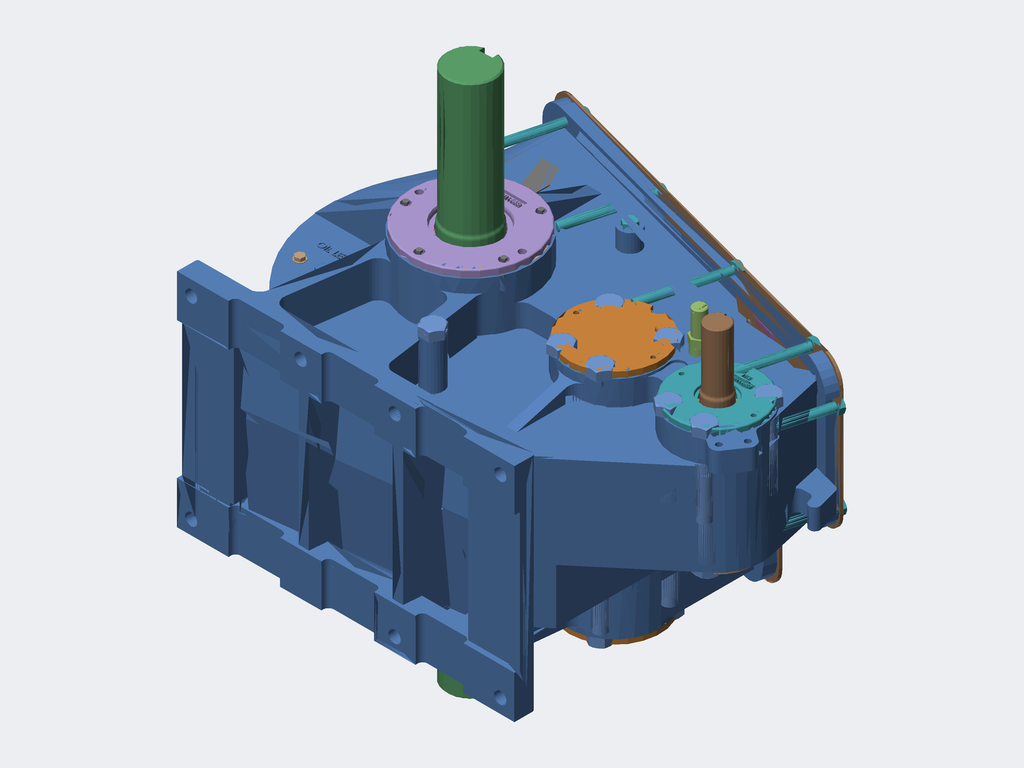Assembly | SolidWorks | 40 different items | 65 placed
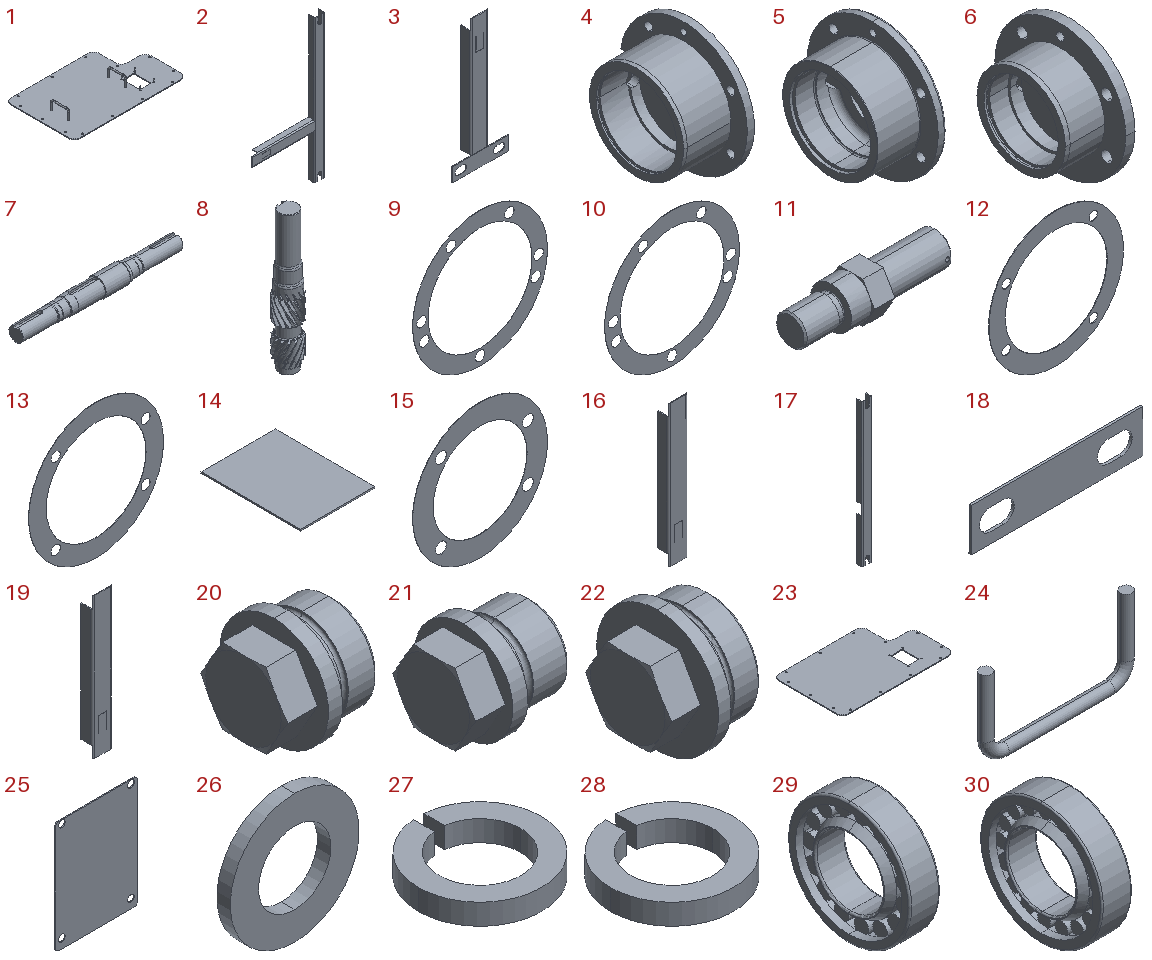Parts list (item | name | quantity | parent item | size | volume | features):
1 | (subassembly) | x1 | - | 998 x 614.68 x 100.025 mm | 3517076 mm3 | -
2 | (subassembly) | x1 | - | 230.1 x 20.55 x 457.2 mm | 62726 mm3 | -
3 | (subassembly) | x1 | - | 101.6 x 20.574 x 241.3 mm | 23948 mm3 | -
4 | - | x2 | - | 95.25 x 221.134 x 222.25 mm | 1161416 mm3 | features ICE 3, HoleWzd 2, Fillet 1, Revolution 1
5 | - | x1 | - | 80.975 x 209.55 x 209.55 mm | 817016 mm3 | features Fillet 5, ICE 5, Chamfer 2, HoleWzd 2, 3DProfileFeature 1, MirrorPattern 1, Revolution 1
6 | - | x1 | - | 65.862 x 177.8 x 177.8 mm | 542990 mm3 | features HoleWzd 2, ICE 2, Fillet 1, Revolution 1
7 | - | x1 | - | 1314 x 152.146 x 152.146 mm | 17037047 mm3 | features Fillet 2, ICE 2, Chamfer 1, Revolution 1
8 | - | x1 | - | 77.902 x 77.902 x 438.15 mm | 1338068 mm3 | features ICE 5, Chamfer 2, CirPattern 2, Helix 2, SweepCut 2, Extrusion 1, Fillet 1, MirrorSolid 1, RefAxis 1, Revolution 1
9 | - | x1 | - | 292.1 x 0.254 x 292.1 mm | 6277 mm3 | features HoleWzd 2, Extrusion 1, MirrorPattern 1
10 | - | x1 | - | 292.1 x 0.1778 x 292.1 mm | 4394 mm3 | features HoleWzd 2, Extrusion 1, MirrorPattern 1
11 | - | x1 | - | 136.144 x 43.994 x 38.1 mm | 113370 mm3 | features ICE 2, Chamfer 1, Fillet 1, Revolution 1
12 | - | x2 | - | 222.25 x 0.7938 x 222.25 mm | 12605 mm3 | features HoleWzd 2, 3DProfileFeature 1, Extrusion 1, MirrorPattern 1
13 | - | x1 | - | 209.55 x 0.381 x 209.55 mm | 5665 mm3 | features 3DProfileFeature 1, Extrusion 1, HoleWzd 1, MirrorPattern 1
14 | - | x1 | - | 101.6 x 136.525 x 2 mm | 27742 mm3 | features Extrusion 1
15 | - | x1 | - | 177.8 x 0.381 x 177.8 mm | 4618 mm3 | features 3DProfileFeature 1, Extrusion 1, HoleWzd 1, MirrorPattern 1
16 | - | x1 | in 3 | 31.75 x 19.05 x 234.95 mm | 20710 mm3 | features ICE 2, Extrusion 1
17 | - | x1 | in 2 | 31.75 x 19.05 x 457.2 mm | 42632 mm3 | features ICE 2, Extrusion 1, MirrorPattern 1
18 | - | x1 | in 3 | 101.6 x 1.524 x 25.4 mm | 3238 mm3 | features Extrusion 1
19 | - | x1 | in 2 | 31.75 x 19.05 x 228.6 mm | 20094 mm3 | features ICE 2, Extrusion 1
20 | - | x2 | - | 32 x 39 x 39 mm | 25996 mm3 | features Boss 1, Cut 1, Fillet 1, Revolution 1
21 | - | x1 | - | 26 x 26 x 26 mm | 9145 mm3 | features Boss 1, Cut 1, Fillet 1, Revolution 1
22 | - | x1 | - | 33 x 49 x 49 mm | 39818 mm3 | features Boss 1, Cut 1, Fillet 1, Revolution 1
23 | - | x1 | in 1 | 998 x 614.68 x 6.35 mm | 3433932 mm3 | features HoleWzd 2, Extrusion 1
24 | - | x2 | in 1 | 165.1 x 12.7 x 88.9 mm | 38148 mm3 | features Sweep 1
25 | - | x1 | - | 139.7 x 1.575 x 190.5 mm | 41244 mm3 | features Extrusion 1, Fillet 1, HoleWzd 1, LPattern 1
26 | - | x2 | - | 24 x 2.5 x 24 mm | 773.126 mm3 | features Revolution 1
27 | - | x4 | - | 15.372 x 15.344 x 2.6 mm | 261.313 mm3 | features Extrusion 1
28 | - | x15 | - | 18.367 x 18.334 x 3.1 mm | 444.091 mm3 | features Extrusion 1
29 | - | x1 | - | 25 x 100 x 100 mm | 86122 mm3 | features Revolution 3, CirPattern 1
30 | - | x1 | - | 31 x 125 x 125 mm | 173586 mm3 | features Revolution 3, CirPattern 1
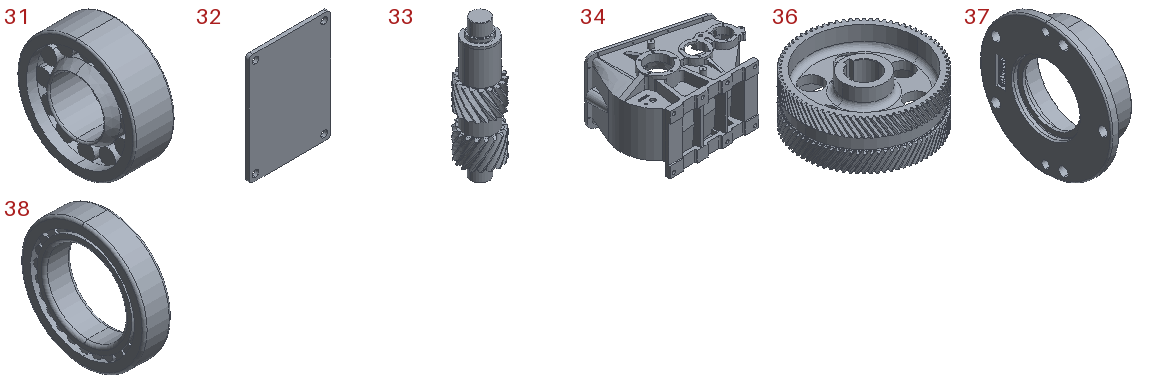31 | - | x2 | - | 48 x 140 x 140 mm | 368578 mm3 | features Revolution 3, CirPattern 1
32 | - | x1 | - | 139.7 x 6.35 x 190.5 mm | 166308 mm3 | features Extrusion 1, Fillet 1, HoleWzd 1, LPattern 1
33 | - | x1 | - | 142.951 x 142.951 x 498.475 mm | 4697605 mm3 | features Chamfer 3, Fillet 2, ICE 2, CirPattern 1, Extrusion 1, Helix 1, MirrorSolid 1, RefAxis 1, Revolution 1, SweepCut 1
34 | - | x1 | - | 1118 x 865.604 x 644.525 mm | 64344550 mm3 | features ICE 78, HoleWzd 17, Fillet 7, 3DProfileFeature 6, RevCut 4, Blend 2, Extrusion 1
35 | - | x1 | - | - | - | features ICE 5, Chamfer 4, Fillet 2, CirPattern 1, Extrusion 1, Helix 1, MirrorSolid 1, RefAxis 1, SweepCut 1
36 | - | x1 | - | 591.617 x 591.617 x 230.532 mm | 20474904 mm3 | features ICE 4, Chamfer 3, Fillet 3, CirPattern 1, Extrusion 1, Helix 1, MirrorSolid 1, RefAxis 1, RevCut 1, SweepCut 1
37 | - | x2 | - | 79.375 x 292.1 x 292.1 mm | 1441408 mm3 | features Fillet 5, ICE 4, HoleWzd 2, Chamfer 1, MirrorPattern 1, Revolution 1
38 | - | x2 | - | 46.04 x 196.8 x 196.8 mm | 612337 mm3 | features Revolution 3, Fillet 2, CirPattern 1
39 | hex bolt_ai | x1 | - | - | - | -
40 | hex nut_ai | x1 | - | - | - | -
Mates (type | each side: item.copy, entity, surface, feature):
In the top assembly
Concentric | 36.1 face cylinder Mirror1 | 7.1 face cylinder Revolve1
Coincident | 36.1 face plane Mirror1 | 7.1 face plane Revolve1
Concentric | 34.1 face cylinder Extrude1 | 7.1 face cylinder Revolve1
Concentric | 33.1 face cylinder Revolve1 | 35.1 face cylinder Extrude6
Coincident | 33.1 face plane Mirror1 | 35.1 face plane Mirror3
Parallel | 33.1 face plane Extrude26 | 35.1 face plane Extrude6
Concentric | 34.1 face cylinder Extrude1 | 33.1 face cylinder Revolve1
Concentric | 33.1 face cylinder Revolve1 | 31.1 face cylinder Base-Revolve
Coincident | 33.1 face plane Revolve1 | 31.1 face plane Base-Revolve
Concentric | 33.1 face cylinder Revolve1 | 31.2 face cylinder Base-Revolve
Tangent | 33.1 face plane Revolve1 | 31.2 face torus Base-Revolve
Concentric | 8.1 face cylinder Revolve1 | 30.1 face cylinder Base-Revolve
Concentric | 8.1 face cylinder Revolve1 | 29.1 face cylinder Base-Revolve
Coincident | 8.1 face plane Mirror1 | 29.1 face plane Base-Revolve
Coincident | 8.1 face plane Extrude5 | 30.1 face plane Base-Revolve
Concentric | 29.1 face cylinder Boss-Revolve2 | 6.1 face cylinder Revolve1
Coincident | 29.1 face plane Boss-Revolve2 | 6.1 face plane Revolve1
Concentric | 30.1 face cylinder Boss-Revolve2 | 5.1 face cylinder Revolve1
Tangent | 30.1 face plane Boss-Revolve2 | 5.1 face torus Fillet2
Concentric | 13.1 face cylinder Boss-Extrude1 | 15.1 face cylinder Boss-Extrude1
Concentric | 6.1 face cylinder Revolve1 | 15.1 face cylinder Boss-Extrude1
Coincident | 5.1 face plane Revolve1 | 13.1 face plane Boss-Extrude1
Coincident | 6.1 face plane Revolve1 | 15.1 face plane Boss-Extrude1
Width | 15.1 face plane Boss-Extrude1 | 13.1 face plane Boss-Extrude1 | 34.1 face plane Extrude42 | 34.1 face plane Extrude60
Concentric | 34.1 face cylinder Extrude1 | 5.1 face cylinder Revolve1
Concentric | 7.1 face cylinder Revolve1 | 38.1 face cylinder Base-Revolve
Concentric | 7.1 face cylinder Revolve1 | 38.2 face cylinder Base-Revolve
Coincident | 7.1 face plane Revolve1 | 38.1 face plane Base-Revolve
Coincident | 7.1 face plane Revolve1 | 38.2 face plane Base-Revolve
Concentric | 7.1 face cylinder Revolve1 | 37.1 face cylinder Revolve1
Concentric | 7.1 face cylinder Revolve1 | 37.2 face cylinder Revolve1
Coincident | 38.1 face plane Boss-Revolve16 | 37.1 face plane Revolve1
Coincident | 38.2 face plane Boss-Revolve16 | 37.2 face plane Revolve1
Coincident | 9.1 edge | 10.1 face cylinder Boss-Extrude1
Concentric | 7.1 face cylinder Revolve1 | 10.1 edge
Coincident | 37.1 face plane Revolve1 | 9.1 face plane Boss-Extrude1
Coincident | 37.2 face plane Revolve1 | 10.1 face plane Boss-Extrude1
Width | 10.1 face plane Boss-Extrude1 | 9.1 face plane Boss-Extrude1 | 34.1 face plane Extrude58 | 34.1 face plane Extrude8
Concentric | 33.1 face cylinder Extrude2 | 4.1 face cylinder Revolve1
Concentric | 31.2 face cylinder Boss-Revolve2 | 4.2 face cylinder Revolve1
Coincident | 31.2 face plane Boss-Revolve2 | 4.2 face plane Revolve1
Coincident | 31.1 face plane Boss-Revolve2 | 4.1 face plane Revolve1
Concentric | 12.1 face cylinder Boss-Extrude1 | 12.2 face cylinder Boss-Extrude1
Concentric | 4.1 face cylinder Revolve1 | 12.2 face cylinder Boss-Extrude1
Coincident | 4.1 face plane Revolve1 | 12.1 face plane Boss-Extrude1
Coincident | 4.2 face plane Revolve1 | 12.2 face plane Boss-Extrude1
Width | 12.2 face plane Boss-Extrude1 | 12.1 face plane Boss-Extrude1 | 34.1 face plane Extrude59 | 34.1 face plane Extrude42
Coincident | 32.1 face plane Boss-Extrude1 | 25.1 face plane Boss-Extrude1 | 3 times
Coincident | 34.1 face plane Extrude1 | 23.1 face plane Extrude1
Concentric | 34.1 face cylinder 1/2-13 Tapped Hole7 | 23.1 face cylinder 9/16 (0.5625) Diameter Hole1 | 2 times
Coincident | 25.1 face plane Boss-Extrude1 | 23.1 face plane Extrude1
Parallel | 32.1 face plane Boss-Extrude1 | 23.1 face plane Extrude1
Coincident | 23.1 face plane Extrude1 | 28.1 face plane Extrude1
Parallel | 34.1 face plane Extrude40 | 37.1 plane
Parallel | 34.1 face plane Extrude40 | 5.1 plane
Parallel | 34.1 face plane Extrude40 | 4.1 plane
Parallel | 34.1 face plane Extrude63 | 37.2 plane
Parallel | 34.1 face plane Extrude63 | 4.2 plane
Parallel | 34.1 face plane Extrude63 | 6.1 plane
Concentric | 34.1 face cylinder 1-1/8-7 Tapped Hole1 | 11.1 face cylinder Revolve1
Coincident | 34.1 face plane Extrude42 | 11.1 face plane Revolve1
Coincident | 26.1 face plane Base-Revolve | 28.2 face plane Extrude1
Concentric | 26.2 face cylinder Base-Revolve | 28.3 face cylinder Extrude1
Coincident | 26.2 face plane Base-Revolve | 28.3 face plane Extrude1
Coincident | 34.1 face plane Extrude52 | 26.2 face plane Base-Revolve
Coincident | 34.1 face plane Extrude46 | 26.1 face plane Base-Revolve
Concentric | 34.1 face cone 1 NPT Tapped Hole1 | 20.1 face cylinder Revolve1
Coincident | 34.1 face plane Extrude50 | 20.1 face plane Revolve1
Concentric | 34.1 face cone 1/2 NPT Tapped Hole1 | 21.1 face cylinder Revolve1
Coincident | 34.1 face plane Extrude4 | 21.1 face plane Revolve1
Concentric | 34.1 face cone Cut-Revolve4 | 20.2 face cylinder Revolve1
Coincident | 34.1 edge | 20.2 face plane Revolve1
Coincident | 34.1 face plane Extrude4 | 22.1 face plane Revolve1
Concentric | 34.1 face cone 1-1/4 NPT Tapped Hole1 | 22.1 face cylinder Revolve1
Coincident | 34.1 face plane Extrude94 | 17.1 face plane Boss-Extrude1
Width | 17.1 face plane Boss-Extrude1 | 17.1 face plane Boss-Extrude1 | 34.1 face plane Extrude1 | 34.1 face plane Extrude2
Width | 17.1 face plane Boss-Extrude1 | 17.1 face plane Boss-Extrude1 | 34.1 face plane Extrude94 | 34.1 face plane Extrude95
Coincident | 34.1 face plane Extrude99 | 18.1 face plane Boss-Extrude1
Width | 16.1 face plane Boss-Extrude1 | 16.1 face plane Boss-Extrude1 | 34.1 face plane Extrude100 | 34.1 face plane Extrude100
DistanceDim | 34.1 face plane Extrude99 | 18.1 face plane Boss-Extrude1
Coincident | 17.1 face plane Boss-Extrude1 | 27.1 face plane Extrude1
Coincident | 17.1 face plane Boss-Extrude1 | 27.2 face plane Extrude1
Coincident | 18.1 face plane Boss-Extrude1 | 27.3 edge
Coincident | 34.1 face plane Extrude1 | 14.1 face plane Extrude1
Parallel | 34.1 face plane Extrude40 | 14.1 face plane Extrude1
In subassembly 1
Coincident | 23.2 face plane Extrude1 | 24.1 face plane Sweep1
Coincident | 23.2 face plane Extrude1 | 24.2 face plane Sweep1
Parallel | 24.2 face cylinder Sweep1 | 24.1 face cylinder Sweep1
DistanceDim | 24.1 axis | 23.2 face plane Extrude1 | 2 times
DistanceDim | 24.2 axis | 24.1 axis
DistanceDim | 24.2 axis | 23.2 face plane Extrude1
In subassembly 2
Coincident | 17.2 face plane Boss-Extrude1 | 19.1 face plane Boss-Extrude1 | 2 times
Coincident | 17.2 face plane Cut-Extrude1 | 19.1 face plane Boss-Extrude1
In subassembly 3
Coincident | 18.2 face plane Boss-Extrude1 | 16.2 face plane Cut-Extrude1
Coincident | 18.2 face plane Boss-Extrude1 | 16.2 face plane Boss-Extrude1
DistanceDim | 16.2 face plane Boss-Extrude1 | 18.2 edge